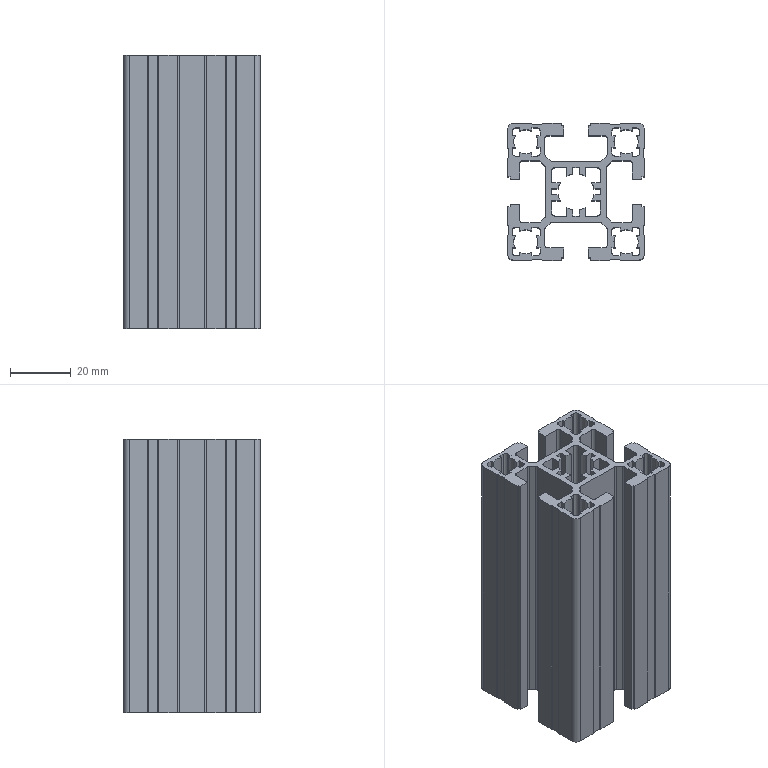Part | STEP file | 4545 profile 3 | 1 solid | 262 faces | box 45 x 45 x 90 mm | volume 62446 mm3 | plane 186 | cylinder 76 | commonest cylinder face diameters 2 x44 8 x20 12 x8 4 x4